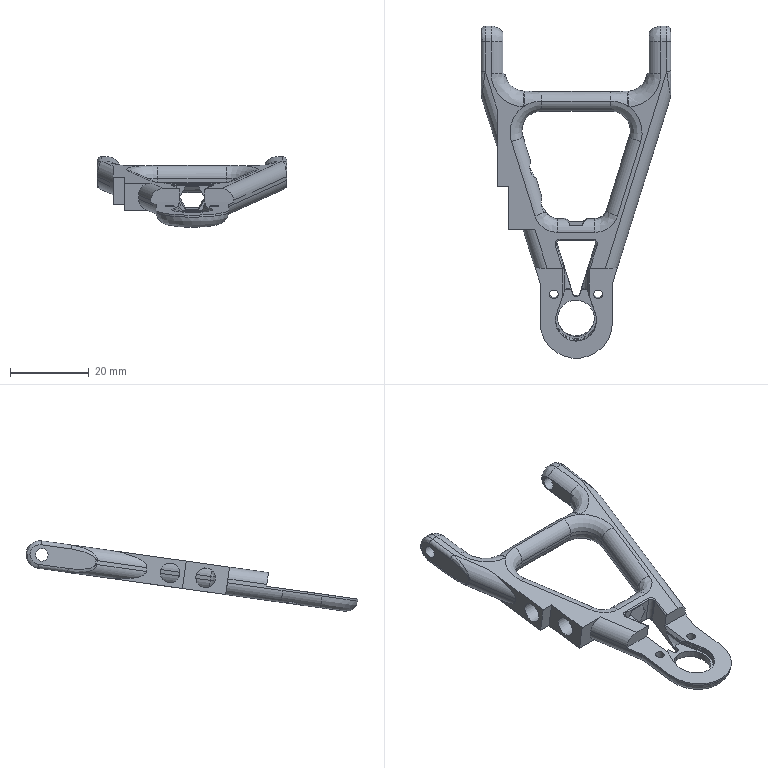Part | STEP file | Zaokr_glenie6 | 1 solid | 154 faces | box 48 x 84.201 x 17.884 mm | volume 7214 mm3 | plane 59 | cylinder 56 | spline 39 | commonest cylinder face diameters 6 x18 2 x10 7 x8 0.6 x6 10 x5 2.2 x2